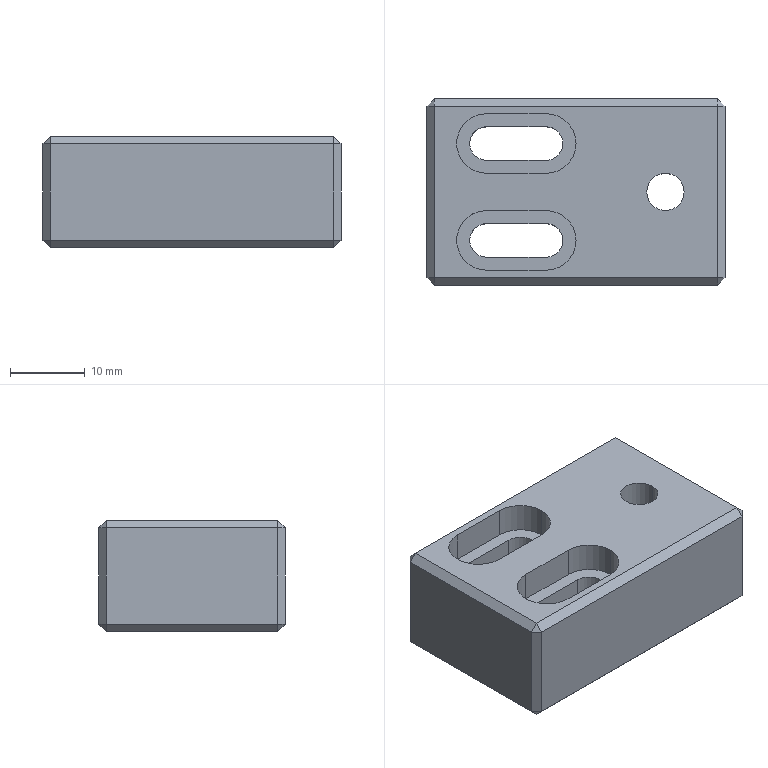Part | STEP file | 04-11 support stop post | 1 solid | 53 faces | box 40 x 25 x 15 mm | volume 11747 mm3 | plane 37 | cylinder 16 | commonest cylinder face diameters 4.5 x6 8 x6 5 x2 12 x2
STEP:
#1=CARTESIAN_POINT('',(-1.75,-6.5,0.));
#2=VERTEX_POINT('',#1);
#3=CARTESIAN_POINT('',(-4.,-4.25,0.));
#4=VERTEX_POINT('',#3);
#5=CARTESIAN_POINT('',(-4.,-6.5,0.));
#6=DIRECTION('',(0.,0.,1.));
#7=DIRECTION('',(1.,0.,0.));
#8=AXIS2_PLACEMENT_3D('',#5,#6,#7);
#9=CIRCLE('',#8,2.25);
#10=EDGE_CURVE('',#2,#4,#9,.T.);
#11=ORIENTED_EDGE('',*,*,#10,.F.);
#12=CARTESIAN_POINT('',(-1.75,-6.5,11.));
#13=VERTEX_POINT('',#12);
#14=CARTESIAN_POINT('',(-1.75,-6.5,-5.));
#15=DIRECTION('',(0.,0.,1.));
#16=VECTOR('',#15,1000.);
#17=LINE('',#14,#16);
#18=EDGE_CURVE('',#2,#13,#17,.T.);
#19=ORIENTED_EDGE('',*,*,#18,.T.);
#20=CARTESIAN_POINT('',(-4.,-4.25,11.));
#21=VERTEX_POINT('',#20);
#22=CARTESIAN_POINT('',(-4.,-6.5,11.));
#23=DIRECTION('',(0.,0.,1.));
#24=DIRECTION('',(-1.,0.,0.));
#25=AXIS2_PLACEMENT_3D('',#22,#23,#24);
#26=CIRCLE('',#25,2.25);
#27=EDGE_CURVE('',#13,#21,#26,.T.);
#28=ORIENTED_EDGE('',*,*,#27,.T.);
#29=CARTESIAN_POINT('',(-4.,-4.25,-5.));
#30=DIRECTION('',(0.,0.,1.));
#31=VECTOR('',#30,1000.);
#32=LINE('',#29,#31);
#33=EDGE_CURVE('',#4,#21,#32,.T.);
#34=ORIENTED_EDGE('',*,*,#33,.F.);
#35=EDGE_LOOP('',(#11,#19,#28,#34));
#36=FACE_OUTER_BOUND('',#35,.T.);
#37=CARTESIAN_POINT('',(-4.,-6.5,-5.));
#38=DIRECTION('',(0.,0.,1.));
#39=DIRECTION('',(1.,0.,0.));
#40=AXIS2_PLACEMENT_3D('',#37,#38,#39);
#41=CYLINDRICAL_SURFACE('',#40,2.25);
#42=ADVANCED_FACE('',(#36),#41,.F.);
#43=CARTESIAN_POINT('',(-1.75,6.5,0.));
#44=VERTEX_POINT('',#43);
#45=CARTESIAN_POINT('',(-4.,8.75,0.));
#46=VERTEX_POINT('',#45);
#47=CARTESIAN_POINT('',(-4.,6.5,0.));
#48=DIRECTION('',(0.,0.,1.));
#49=DIRECTION('',(1.,0.,0.));
#50=AXIS2_PLACEMENT_3D('',#47,#48,#49);
#51=CIRCLE('',#50,2.25);
#52=EDGE_CURVE('',#44,#46,#51,.T.);
#53=ORIENTED_EDGE('',*,*,#52,.F.);
#54=CARTESIAN_POINT('',(-1.75,6.5,11.));
#55=VERTEX_POINT('',#54);
#56=CARTESIAN_POINT('',(-1.75,6.5,-5.));
#57=DIRECTION('',(0.,0.,1.));
#58=VECTOR('',#57,1000.);
#59=LINE('',#56,#58);
#60=EDGE_CURVE('',#44,#55,#59,.T.);
#61=ORIENTED_EDGE('',*,*,#60,.T.);
#62=CARTESIAN_POINT('',(-4.,8.75,11.));
#63=VERTEX_POINT('',#62);
#64=CARTESIAN_POINT('',(-4.,6.5,11.));
#65=DIRECTION('',(0.,0.,1.));
#66=DIRECTION('',(1.,0.,0.));
#67=AXIS2_PLACEMENT_3D('',#64,#65,#66);
#68=CIRCLE('',#67,2.25);
#69=EDGE_CURVE('',#55,#63,#68,.T.);
#70=ORIENTED_EDGE('',*,*,#69,.T.);
#71=CARTESIAN_POINT('',(-4.,8.75,-5.));
#72=DIRECTION('',(0.,0.,1.));
#73=VECTOR('',#72,1000.);
#74=LINE('',#71,#73);
#75=EDGE_CURVE('',#46,#63,#74,.T.);
#76=ORIENTED_EDGE('',*,*,#75,.F.);
#77=EDGE_LOOP('',(#53,#61,#70,#76));
#78=FACE_OUTER_BOUND('',#77,.T.);
#79=CARTESIAN_POINT('',(-4.,6.5,-5.));
#80=DIRECTION('',(0.,0.,1.));
#81=DIRECTION('',(1.,0.,0.));
#82=AXIS2_PLACEMENT_3D('',#79,#80,#81);
#83=CYLINDRICAL_SURFACE('',#82,2.25);
#84=ADVANCED_FACE('',(#78),#83,.F.);
#85=CARTESIAN_POINT('',(0.,-6.5,11.));
#86=VERTEX_POINT('',#85);
#87=CARTESIAN_POINT('',(-4.,-2.5,11.));
#88=VERTEX_POINT('',#87);
#89=CARTESIAN_POINT('',(-4.,-6.5,11.));
#90=DIRECTION('',(0.,0.,1.));
#91=DIRECTION('',(-1.,0.,0.));
#92=AXIS2_PLACEMENT_3D('',#89,#90,#91);
#93=CIRCLE('',#92,4.);
#94=EDGE_CURVE('',#86,#88,#93,.T.);
#95=ORIENTED_EDGE('',*,*,#94,.F.);
#96=CARTESIAN_POINT('',(0.,-6.5,15.));
#97=VERTEX_POINT('',#96);
#98=CARTESIAN_POINT('',(0.,-6.5,11.));
#99=DIRECTION('',(0.,0.,1.));
#100=VECTOR('',#99,1000.);
#101=LINE('',#98,#100);
#102=EDGE_CURVE('',#86,#97,#101,.T.);
#103=ORIENTED_EDGE('',*,*,#102,.T.);
#104=CARTESIAN_POINT('',(-4.,-2.5,15.));
#105=VERTEX_POINT('',#104);
#106=CARTESIAN_POINT('',(-4.,-6.5,15.));
#107=DIRECTION('',(0.,0.,1.));
#108=DIRECTION('',(-1.,0.,0.));
#109=AXIS2_PLACEMENT_3D('',#106,#107,#108);
#110=CIRCLE('',#109,4.);
#111=EDGE_CURVE('',#97,#105,#110,.T.);
#112=ORIENTED_EDGE('',*,*,#111,.T.);
#113=CARTESIAN_POINT('',(-4.,-2.5,11.));
#114=DIRECTION('',(0.,0.,1.));
#115=VECTOR('',#114,1000.);
#116=LINE('',#113,#115);
#117=EDGE_CURVE('',#88,#105,#116,.T.);
#118=ORIENTED_EDGE('',*,*,#117,.F.);
#119=EDGE_LOOP('',(#95,#103,#112,#118));
#120=FACE_OUTER_BOUND('',#119,.T.);
#121=CARTESIAN_POINT('',(-4.,-6.5,11.));
#122=DIRECTION('',(0.,0.,1.));
#123=DIRECTION('',(1.,0.,0.));
#124=AXIS2_PLACEMENT_3D('',#121,#122,#123);
#125=CYLINDRICAL_SURFACE('',#124,4.);
#126=ADVANCED_FACE('',(#120),#125,.F.);
#127=CARTESIAN_POINT('',(0.,6.5,11.));
#128=VERTEX_POINT('',#127);
#129=CARTESIAN_POINT('',(-4.,10.5,11.));
#130=VERTEX_POINT('',#129);
#131=CARTESIAN_POINT('',(-4.,6.5,11.));
#132=DIRECTION('',(0.,0.,1.));
#133=DIRECTION('',(1.,0.,0.));
#134=AXIS2_PLACEMENT_3D('',#131,#132,#133);
#135=CIRCLE('',#134,4.);
#136=EDGE_CURVE('',#128,#130,#135,.T.);
#137=ORIENTED_EDGE('',*,*,#136,.F.);
#138=CARTESIAN_POINT('',(0.,6.5,15.));
#139=VERTEX_POINT('',#138);
#140=CARTESIAN_POINT('',(0.,6.5,11.));
#141=DIRECTION('',(0.,0.,1.));
#142=VECTOR('',#141,1000.);
#143=LINE('',#140,#142);
#144=EDGE_CURVE('',#128,#139,#143,.T.);
#145=ORIENTED_EDGE('',*,*,#144,.T.);
#146=CARTESIAN_POINT('',(-4.,10.5,15.));
#147=VERTEX_POINT('',#146);
#148=CARTESIAN_POINT('',(-4.,6.5,15.));
#149=DIRECTION('',(0.,0.,1.));
#150=DIRECTION('',(1.,0.,0.));
#151=AXIS2_PLACEMENT_3D('',#148,#149,#150);
#152=CIRCLE('',#151,4.);
#153=EDGE_CURVE('',#139,#147,#152,.T.);
#154=ORIENTED_EDGE('',*,*,#153,.T.);
#155=CARTESIAN_POINT('',(-4.,10.5,11.));
#156=DIRECTION('',(0.,0.,1.));
#157=VECTOR('',#156,1000.);
#158=LINE('',#155,#157);
#159=EDGE_CURVE('',#130,#147,#158,.T.);
#160=ORIENTED_EDGE('',*,*,#159,.F.);
#161=EDGE_LOOP('',(#137,#145,#154,#160));
#162=FACE_OUTER_BOUND('',#161,.T.);
#163=CARTESIAN_POINT('',(-4.,6.5,11.));
#164=DIRECTION('',(0.,0.,1.));
#165=DIRECTION('',(1.,0.,0.));
#166=AXIS2_PLACEMENT_3D('',#163,#164,#165);
#167=CYLINDRICAL_SURFACE('',#166,4.);
#168=ADVANCED_FACE('',(#162),#167,.F.);
#169=CARTESIAN_POINT('',(18.,0.,8.));
#170=VERTEX_POINT('',#169);
#171=CARTESIAN_POINT('',(6.,0.,8.));
#172=VERTEX_POINT('',#171);
#173=CARTESIAN_POINT('',(12.,0.,8.));
#174=DIRECTION('',(0.,0.,-1.));
#175=DIRECTION('',(-1.,0.,0.));
#176=AXIS2_PLACEMENT_3D('',#173,#174,#175);
#177=CIRCLE('',#176,6.);
#178=EDGE_CURVE('',#170,#172,#177,.T.);
#179=ORIENTED_EDGE('',*,*,#178,.F.);
#180=CARTESIAN_POINT('',(18.,0.,0.));
#181=VERTEX_POINT('',#180);
#182=CARTESIAN_POINT('',(18.,0.,8.));
#183=DIRECTION('',(0.,0.,-1.));
#184=VECTOR('',#183,1000.);
#185=LINE('',#182,#184);
#186=EDGE_CURVE('',#170,#181,#185,.T.);
#187=ORIENTED_EDGE('',*,*,#186,.T.);
#188=CARTESIAN_POINT('',(6.,0.,0.));
#189=VERTEX_POINT('',#188);
#190=CARTESIAN_POINT('',(12.,0.,0.));
#191=DIRECTION('',(0.,0.,-1.));
#192=DIRECTION('',(-1.,0.,0.));
#193=AXIS2_PLACEMENT_3D('',#190,#191,#192);
#194=CIRCLE('',#193,6.);
#195=EDGE_CURVE('',#181,#189,#194,.T.);
#196=ORIENTED_EDGE('',*,*,#195,.T.);
#197=CARTESIAN_POINT('',(6.,0.,8.));
#198=DIRECTION('',(0.,0.,-1.));
#199=VECTOR('',#198,1000.);
#200=LINE('',#197,#199);
#201=EDGE_CURVE('',#172,#189,#200,.T.);
#202=ORIENTED_EDGE('',*,*,#201,.F.);
#203=EDGE_LOOP('',(#179,#187,#196,#202));
#204=FACE_OUTER_BOUND('',#203,.T.);
#205=CARTESIAN_POINT('',(12.,0.,8.));
#206=DIRECTION('',(0.,0.,-1.));
#207=DIRECTION('',(-1.,0.,0.));
#208=AXIS2_PLACEMENT_3D('',#205,#206,#207);
#209=CYLINDRICAL_SURFACE('',#208,6.);
#210=ADVANCED_FACE('',(#204),#209,.F.);
#211=CARTESIAN_POINT('',(9.5,0.,8.));
#212=VERTEX_POINT('',#211);
#213=CARTESIAN_POINT('',(14.5,0.,8.));
#214=VERTEX_POINT('',#213);
#215=CARTESIAN_POINT('',(12.,0.,8.));
#216=DIRECTION('',(0.,0.,1.));
#217=DIRECTION('',(-1.,0.,0.));
#218=AXIS2_PLACEMENT_3D('',#215,#216,#217);
#219=CIRCLE('',#218,2.5);
#220=EDGE_CURVE('',#212,#214,#219,.T.);
#221=ORIENTED_EDGE('',*,*,#220,.F.);
#222=CARTESIAN_POINT('',(9.5,0.,15.));
#223=VERTEX_POINT('',#222);
#224=CARTESIAN_POINT('',(9.5,0.,-2.));
#225=DIRECTION('',(0.,0.,1.));
#226=VECTOR('',#225,1000.);
#227=LINE('',#224,#226);
#228=EDGE_CURVE('',#212,#223,#227,.T.);
#229=ORIENTED_EDGE('',*,*,#228,.T.);
#230=CARTESIAN_POINT('',(14.5,0.,15.));
#231=VERTEX_POINT('',#230);
#232=CARTESIAN_POINT('',(12.,0.,15.));
#233=DIRECTION('',(0.,0.,1.));
#234=DIRECTION('',(1.,0.,0.));
#235=AXIS2_PLACEMENT_3D('',#232,#233,#234);
#236=CIRCLE('',#235,2.5);
#237=EDGE_CURVE('',#223,#231,#236,.T.);
#238=ORIENTED_EDGE('',*,*,#237,.T.);
#239=CARTESIAN_POINT('',(14.5,0.,-2.));
#240=DIRECTION('',(0.,0.,1.));
#241=VECTOR('',#240,1000.);
#242=LINE('',#239,#241);
#243=EDGE_CURVE('',#214,#231,#242,.T.);
#244=ORIENTED_EDGE('',*,*,#243,.F.);
#245=EDGE_LOOP('',(#221,#229,#238,#244));
#246=FACE_OUTER_BOUND('',#245,.T.);
#247=CARTESIAN_POINT('',(12.,0.,-2.));
#248=DIRECTION('',(0.,0.,1.));
#249=DIRECTION('',(1.,0.,0.));
#250=AXIS2_PLACEMENT_3D('',#247,#248,#249);
#251=CYLINDRICAL_SURFACE('',#250,2.5);
#252=ADVANCED_FACE('',(#246),#251,.F.);
#253=ORIENTED_EDGE('',*,*,#228,.F.);
#254=CARTESIAN_POINT('',(12.,0.,8.));
#255=DIRECTION('',(0.,0.,1.));
#256=DIRECTION('',(-1.,0.,0.));
#257=AXIS2_PLACEMENT_3D('',#254,#255,#256);
#258=CIRCLE('',#257,2.5);
#259=EDGE_CURVE('',#214,#212,#258,.T.);
#260=ORIENTED_EDGE('',*,*,#259,.F.);
#261=ORIENTED_EDGE('',*,*,#243,.T.);
#262=CARTESIAN_POINT('',(12.,0.,15.));
#263=DIRECTION('',(0.,0.,1.));
#264=DIRECTION('',(1.,0.,0.));
#265=AXIS2_PLACEMENT_3D('',#262,#263,#264);
#266=CIRCLE('',#265,2.5);
#267=EDGE_CURVE('',#231,#223,#266,.T.);
#268=ORIENTED_EDGE('',*,*,#267,.T.);
#269=EDGE_LOOP('',(#253,#260,#261,#268));
#270=FACE_OUTER_BOUND('',#269,.T.);
#271=CARTESIAN_POINT('',(12.,0.,-2.));
#272=DIRECTION('',(0.,0.,1.));
#273=DIRECTION('',(1.,0.,0.));
#274=AXIS2_PLACEMENT_3D('',#271,#272,#273);
#275=CYLINDRICAL_SURFACE('',#274,2.5);
#276=ADVANCED_FACE('',(#270),#275,.F.);
#277=CARTESIAN_POINT('',(20.,11.5,14.));
#278=VERTEX_POINT('',#277);
#279=CARTESIAN_POINT('',(20.,-11.5,14.));
#280=VERTEX_POINT('',#279);
#281=CARTESIAN_POINT('',(20.,-12.5,14.));
#282=DIRECTION('',(0.,-1.,0.));
#283=VECTOR('',#282,1000.);
#284=LINE('',#281,#283);
#285=EDGE_CURVE('',#278,#280,#284,.T.);
#286=ORIENTED_EDGE('',*,*,#285,.T.);
#287=CARTESIAN_POINT('',(20.,-11.5,1.));
#288=VERTEX_POINT('',#287);
#289=CARTESIAN_POINT('',(20.,-11.5,15.));
#290=DIRECTION('',(0.,0.,-1.));
#291=VECTOR('',#290,1000.);
#292=LINE('',#289,#291);
#293=EDGE_CURVE('',#280,#288,#292,.T.);
#294=ORIENTED_EDGE('',*,*,#293,.T.);
#295=CARTESIAN_POINT('',(20.,11.5,1.));
#296=VERTEX_POINT('',#295);
#297=CARTESIAN_POINT('',(20.,12.5,1.));
#298=DIRECTION('',(0.,1.,0.));
#299=VECTOR('',#298,1000.);
#300=LINE('',#297,#299);
#301=EDGE_CURVE('',#288,#296,#300,.T.);
#302=ORIENTED_EDGE('',*,*,#301,.T.);
#303=CARTESIAN_POINT('',(20.,11.5,15.));
#304=DIRECTION('',(0.,0.,1.));
#305=VECTOR('',#304,1000.);
#306=LINE('',#303,#305);
#307=EDGE_CURVE('',#296,#278,#306,.T.);
#308=ORIENTED_EDGE('',*,*,#307,.T.);
#309=EDGE_LOOP('',(#286,#294,#302,#308));
#310=FACE_OUTER_BOUND('',#309,.T.);
#311=CARTESIAN_POINT('',(20.,12.5,15.));
#312=DIRECTION('',(-1.,0.,0.));
#313=DIRECTION('',(0.,-1.,0.));
#314=AXIS2_PLACEMENT_3D('',#311,#312,#313);
#315=PLANE('',#314);
#316=ADVANCED_FACE('',(#310),#315,.F.);
#317=CARTESIAN_POINT('',(19.,12.5,14.));
#318=VERTEX_POINT('',#317);
#319=CARTESIAN_POINT('',(19.,12.5,1.));
#320=VERTEX_POINT('',#319);
#321=CARTESIAN_POINT('',(19.,12.5,15.));
#322=DIRECTION('',(0.,0.,-1.));
#323=VECTOR('',#322,1000.);
#324=LINE('',#321,#323);
#325=EDGE_CURVE('',#318,#320,#324,.T.);
#326=ORIENTED_EDGE('',*,*,#325,.T.);
#327=CARTESIAN_POINT('',(-19.,12.5,1.));
#328=VERTEX_POINT('',#327);
#329=CARTESIAN_POINT('',(-20.,12.5,1.));
#330=DIRECTION('',(-1.,0.,0.));
#331=VECTOR('',#330,1000.);
#332=LINE('',#329,#331);
#333=EDGE_CURVE('',#320,#328,#332,.T.);
#334=ORIENTED_EDGE('',*,*,#333,.T.);
#335=CARTESIAN_POINT('',(-19.,12.5,14.));
#336=VERTEX_POINT('',#335);
#337=CARTESIAN_POINT('',(-19.,12.5,15.));
#338=DIRECTION('',(0.,0.,1.));
#339=VECTOR('',#338,1000.);
#340=LINE('',#337,#339);
#341=EDGE_CURVE('',#328,#336,#340,.T.);
#342=ORIENTED_EDGE('',*,*,#341,.T.);
#343=CARTESIAN_POINT('',(20.,12.5,14.));
#344=DIRECTION('',(1.,0.,0.));
#345=VECTOR('',#344,1000.);
#346=LINE('',#343,#345);
#347=EDGE_CURVE('',#336,#318,#346,.T.);
#348=ORIENTED_EDGE('',*,*,#347,.T.);
#349=EDGE_LOOP('',(#326,#334,#342,#348));
#350=FACE_OUTER_BOUND('',#349,.T.);
#351=CARTESIAN_POINT('',(-20.,12.5,15.));
#352=DIRECTION('',(0.,-1.,0.));
#353=DIRECTION('',(0.,0.,-1.));
#354=AXIS2_PLACEMENT_3D('',#351,#352,#353);
#355=PLANE('',#354);
#356=ADVANCED_FACE('',(#350),#355,.F.);
#357=CARTESIAN_POINT('',(-20.,11.5,14.));
#358=VERTEX_POINT('',#357);
#359=CARTESIAN_POINT('',(-20.,11.5,1.));
#360=VERTEX_POINT('',#359);
#361=CARTESIAN_POINT('',(-20.,11.5,15.));
#362=DIRECTION('',(0.,0.,-1.));
#363=VECTOR('',#362,1000.);
#364=LINE('',#361,#363);
#365=EDGE_CURVE('',#358,#360,#364,.T.);
#366=ORIENTED_EDGE('',*,*,#365,.T.);
#367=CARTESIAN_POINT('',(-20.,-11.5,1.));
#368=VERTEX_POINT('',#367);
#369=CARTESIAN_POINT('',(-20.,12.5,1.));
#370=DIRECTION('',(0.,-1.,0.));
#371=VECTOR('',#370,1000.);
#372=LINE('',#369,#371);
#373=EDGE_CURVE('',#360,#368,#372,.T.);
#374=ORIENTED_EDGE('',*,*,#373,.T.);
#375=CARTESIAN_POINT('',(-20.,-11.5,14.));
#376=VERTEX_POINT('',#375);
#377=CARTESIAN_POINT('',(-20.,-11.5,15.));
#378=DIRECTION('',(0.,0.,1.));
#379=VECTOR('',#378,1000.);
#380=LINE('',#377,#379);
#381=EDGE_CURVE('',#368,#376,#380,.T.);
#382=ORIENTED_EDGE('',*,*,#381,.T.);
#383=CARTESIAN_POINT('',(-20.,12.5,14.));
#384=DIRECTION('',(0.,1.,0.));
#385=VECTOR('',#384,1000.);
#386=LINE('',#383,#385);
#387=EDGE_CURVE('',#376,#358,#386,.T.);
#388=ORIENTED_EDGE('',*,*,#387,.T.);
#389=EDGE_LOOP('',(#366,#374,#382,#388));
#390=FACE_OUTER_BOUND('',#389,.T.);
#391=CARTESIAN_POINT('',(-20.,12.5,15.));
#392=DIRECTION('',(1.,0.,0.));
#393=DIRECTION('',(0.,1.,0.));
#394=AXIS2_PLACEMENT_3D('',#391,#392,#393);
#395=PLANE('',#394);
#396=ADVANCED_FACE('',(#390),#395,.F.);
#397=CARTESIAN_POINT('',(19.,-12.5,1.));
#398=VERTEX_POINT('',#397);
#399=CARTESIAN_POINT('',(19.,-12.5,14.));
#400=VERTEX_POINT('',#399);
#401=CARTESIAN_POINT('',(19.,-12.5,15.));
#402=DIRECTION('',(0.,0.,1.));
#403=VECTOR('',#402,1000.);
#404=LINE('',#401,#403);
#405=EDGE_CURVE('',#398,#400,#404,.T.);
#406=ORIENTED_EDGE('',*,*,#405,.T.);
#407=CARTESIAN_POINT('',(-19.,-12.5,14.));
#408=VERTEX_POINT('',#407);
#409=CARTESIAN_POINT('',(-20.,-12.5,14.));
#410=DIRECTION('',(-1.,0.,0.));
#411=VECTOR('',#410,1000.);
#412=LINE('',#409,#411);
#413=EDGE_CURVE('',#400,#408,#412,.T.);
#414=ORIENTED_EDGE('',*,*,#413,.T.);
#415=CARTESIAN_POINT('',(-19.,-12.5,1.));
#416=VERTEX_POINT('',#415);
#417=CARTESIAN_POINT('',(-19.,-12.5,15.));
#418=DIRECTION('',(0.,0.,-1.));
#419=VECTOR('',#418,1000.);
#420=LINE('',#417,#419);
#421=EDGE_CURVE('',#408,#416,#420,.T.);
#422=ORIENTED_EDGE('',*,*,#421,.T.);
#423=CARTESIAN_POINT('',(-20.,-12.5,1.));
#424=DIRECTION('',(1.,0.,0.));
#425=VECTOR('',#424,1000.);
#426=LINE('',#423,#425);
#427=EDGE_CURVE('',#416,#398,#426,.T.);
#428=ORIENTED_EDGE('',*,*,#427,.T.);
#429=EDGE_LOOP('',(#406,#414,#422,#428));
#430=FACE_OUTER_BOUND('',#429,.T.);
#431=CARTESIAN_POINT('',(-20.,-12.5,15.));
#432=DIRECTION('',(0.,1.,0.));
#433=DIRECTION('',(0.,0.,1.));
#434=AXIS2_PLACEMENT_3D('',#431,#432,#433);
#435=PLANE('',#434);
#436=ADVANCED_FACE('',(#430),#435,.F.);
#437=CARTESIAN_POINT('',(-19.,11.5,15.));
#438=VERTEX_POINT('',#437);
#439=CARTESIAN_POINT('',(-19.,-11.5,15.));
#440=VERTEX_POINT('',#439);
#441=CARTESIAN_POINT('',(-19.,-12.5,15.));
#442=DIRECTION('',(0.,-1.,0.));
#443=VECTOR('',#442,1000.);
#444=LINE('',#441,#443);
#445=EDGE_CURVE('',#438,#440,#444,.T.);
#446=ORIENTED_EDGE('',*,*,#445,.T.);
#447=CARTESIAN_POINT('',(19.,-11.5,15.));
#448=VERTEX_POINT('',#447);
#449=CARTESIAN_POINT('',(20.,-11.5,15.));
#450=DIRECTION('',(1.,0.,0.));
#451=VECTOR('',#450,1000.);
#452=LINE('',#449,#451);
#453=EDGE_CURVE('',#440,#448,#452,.T.);
#454=ORIENTED_EDGE('',*,*,#453,.T.);
#455=CARTESIAN_POINT('',(19.,11.5,15.));
#456=VERTEX_POINT('',#455);
#457=CARTESIAN_POINT('',(19.,12.5,15.));
#458=DIRECTION('',(0.,1.,0.));
#459=VECTOR('',#458,1000.);
#460=LINE('',#457,#459);
#461=EDGE_CURVE('',#448,#456,#460,.T.);
#462=ORIENTED_EDGE('',*,*,#461,.T.);
#463=CARTESIAN_POINT('',(-20.,11.5,15.));
#464=DIRECTION('',(-1.,0.,0.));
#465=VECTOR('',#464,1000.);
#466=LINE('',#463,#465);
#467=EDGE_CURVE('',#456,#438,#466,.T.);
#468=ORIENTED_EDGE('',*,*,#467,.T.);
#469=EDGE_LOOP('',(#446,#454,#462,#468));
#470=FACE_OUTER_BOUND('',#469,.T.);
#471=CARTESIAN_POINT('',(-12.,-2.5,15.));
#472=VERTEX_POINT('',#471);
#473=CARTESIAN_POINT('',(-12.,-10.5,15.));
#474=VERTEX_POINT('',#473);
#475=CARTESIAN_POINT('',(-12.,-6.5,15.));
#476=DIRECTION('',(0.,0.,1.));
#477=DIRECTION('',(-1.,0.,0.));
#478=AXIS2_PLACEMENT_3D('',#475,#476,#477);
#479=CIRCLE('',#478,4.);
#480=EDGE_CURVE('',#472,#474,#479,.T.);
#481=ORIENTED_EDGE('',*,*,#480,.F.);
#482=CARTESIAN_POINT('',(-12.,-2.5,15.));
#483=DIRECTION('',(-1.,0.,0.));
#484=VECTOR('',#483,1000.);
#485=LINE('',#482,#484);
#486=EDGE_CURVE('',#105,#472,#485,.T.);
#487=ORIENTED_EDGE('',*,*,#486,.F.);
#488=ORIENTED_EDGE('',*,*,#111,.F.);
#489=CARTESIAN_POINT('',(-4.,-10.5,15.));
#490=VERTEX_POINT('',#489);
#491=CARTESIAN_POINT('',(-4.,-6.5,15.));
#492=DIRECTION('',(0.,0.,1.));
#493=DIRECTION('',(-1.,0.,0.));
#494=AXIS2_PLACEMENT_3D('',#491,#492,#493);
#495=CIRCLE('',#494,4.);
#496=EDGE_CURVE('',#490,#97,#495,.T.);
#497=ORIENTED_EDGE('',*,*,#496,.F.);
#498=CARTESIAN_POINT('',(-12.,-10.5,15.));
#499=DIRECTION('',(1.,0.,0.));
#500=VECTOR('',#499,1000.);
#501=LINE('',#498,#500);
#502=EDGE_CURVE('',#474,#490,#501,.T.);
#503=ORIENTED_EDGE('',*,*,#502,.F.);
#504=EDGE_LOOP('',(#481,#487,#488,#497,#503));
#505=FACE_BOUND('',#504,.T.);
#506=CARTESIAN_POINT('',(-12.,10.5,15.));
#507=VERTEX_POINT('',#506);
#508=CARTESIAN_POINT('',(-12.,2.5,15.));
#509=VERTEX_POINT('',#508);
#510=CARTESIAN_POINT('',(-12.,6.5,15.));
#511=DIRECTION('',(0.,0.,1.));
#512=DIRECTION('',(1.,0.,0.));
#513=AXIS2_PLACEMENT_3D('',#510,#511,#512);
#514=CIRCLE('',#513,4.);
#515=EDGE_CURVE('',#507,#509,#514,.T.);
#516=ORIENTED_EDGE('',*,*,#515,.F.);
#517=CARTESIAN_POINT('',(-12.,10.5,15.));
#518=DIRECTION('',(-1.,0.,0.));
#519=VECTOR('',#518,1000.);
#520=LINE('',#517,#519);
#521=EDGE_CURVE('',#147,#507,#520,.T.);
#522=ORIENTED_EDGE('',*,*,#521,.F.);
#523=ORIENTED_EDGE('',*,*,#153,.F.);
#524=CARTESIAN_POINT('',(-4.,2.5,15.));
#525=VERTEX_POINT('',#524);
#526=CARTESIAN_POINT('',(-4.,6.5,15.));
#527=DIRECTION('',(0.,0.,1.));
#528=DIRECTION('',(1.,0.,0.));
#529=AXIS2_PLACEMENT_3D('',#526,#527,#528);
#530=CIRCLE('',#529,4.);
#531=EDGE_CURVE('',#525,#139,#530,.T.);
#532=ORIENTED_EDGE('',*,*,#531,.F.);
#533=CARTESIAN_POINT('',(-12.,2.5,15.));
#534=DIRECTION('',(1.,0.,0.));
#535=VECTOR('',#534,1000.);
#536=LINE('',#533,#535);
#537=EDGE_CURVE('',#509,#525,#536,.T.);
#538=ORIENTED_EDGE('',*,*,#537,.F.);
#539=EDGE_LOOP('',(#516,#522,#523,#532,#538));
#540=FACE_BOUND('',#539,.T.);
#541=ORIENTED_EDGE('',*,*,#267,.F.);
#542=ORIENTED_EDGE('',*,*,#237,.F.);
#543=EDGE_LOOP('',(#541,#542));
#544=FACE_BOUND('',#543,.T.);
#545=CARTESIAN_POINT('',(20.,-12.5,15.));
#546=DIRECTION('',(0.,0.,1.));
#547=DIRECTION('',(1.,0.,0.));
#548=AXIS2_PLACEMENT_3D('',#545,#546,#547);
#549=PLANE('',#548);
#550=ADVANCED_FACE('',(#470,#505,#540,#544),#549,.T.);
#551=CARTESIAN_POINT('',(19.,11.5,0.));
#552=VERTEX_POINT('',#551);
#553=CARTESIAN_POINT('',(19.,-11.5,0.));
#554=VERTEX_POINT('',#553);
#555=CARTESIAN_POINT('',(19.,-12.5,0.));
#556=DIRECTION('',(0.,-1.,0.));
#557=VECTOR('',#556,1000.);
#558=LINE('',#555,#557);
#559=EDGE_CURVE('',#552,#554,#558,.T.);
#560=ORIENTED_EDGE('',*,*,#559,.T.);
#561=CARTESIAN_POINT('',(-19.,-11.5,0.));
#562=VERTEX_POINT('',#561);
#563=CARTESIAN_POINT('',(20.,-11.5,0.));
#564=DIRECTION('',(-1.,0.,0.));
#565=VECTOR('',#564,1000.);
#566=LINE('',#563,#565);
#567=EDGE_CURVE('',#554,#562,#566,.T.);
#568=ORIENTED_EDGE('',*,*,#567,.T.);
#569=CARTESIAN_POINT('',(-19.,11.5,0.));
#570=VERTEX_POINT('',#569);
#571=CARTESIAN_POINT('',(-19.,-12.5,0.));
#572=DIRECTION('',(0.,1.,0.));
#573=VECTOR('',#572,1000.);
#574=LINE('',#571,#573);
#575=EDGE_CURVE('',#562,#570,#574,.T.);
#576=ORIENTED_EDGE('',*,*,#575,.T.);
#577=CARTESIAN_POINT('',(20.,11.5,0.));
#578=DIRECTION('',(1.,0.,0.));
#579=VECTOR('',#578,1000.);
#580=LINE('',#577,#579);
#581=EDGE_CURVE('',#570,#552,#580,.T.);
#582=ORIENTED_EDGE('',*,*,#581,.T.);
#583=EDGE_LOOP('',(#560,#568,#576,#582));
#584=FACE_OUTER_BOUND('',#583,.T.);
#585=CARTESIAN_POINT('',(-12.,-4.25,0.));
#586=VERTEX_POINT('',#585);
#587=CARTESIAN_POINT('',(20.,-4.25,0.));
#588=DIRECTION('',(-1.,0.,0.));
#589=VECTOR('',#588,1000.);
#590=LINE('',#587,#589);
#591=EDGE_CURVE('',#4,#586,#590,.T.);
#592=ORIENTED_EDGE('',*,*,#591,.T.);
#593=CARTESIAN_POINT('',(-12.,-8.75,0.));
#594=VERTEX_POINT('',#593);
#595=CARTESIAN_POINT('',(-12.,-6.5,0.));
#596=DIRECTION('',(0.,0.,1.));
#597=DIRECTION('',(1.,0.,0.));
#598=AXIS2_PLACEMENT_3D('',#595,#596,#597);
#599=CIRCLE('',#598,2.25);
#600=EDGE_CURVE('',#586,#594,#599,.T.);
#601=ORIENTED_EDGE('',*,*,#600,.T.);
#602=CARTESIAN_POINT('',(-4.,-8.75,0.));
#603=VERTEX_POINT('',#602);
#604=CARTESIAN_POINT('',(20.,-8.75,0.));
#605=DIRECTION('',(1.,0.,0.));
#606=VECTOR('',#605,1000.);
#607=LINE('',#604,#606);
#608=EDGE_CURVE('',#594,#603,#607,.T.);
#609=ORIENTED_EDGE('',*,*,#608,.T.);
#610=CARTESIAN_POINT('',(-4.,-6.5,0.));
#611=DIRECTION('',(0.,0.,1.));
#612=DIRECTION('',(1.,0.,0.));
#613=AXIS2_PLACEMENT_3D('',#610,#611,#612);
#614=CIRCLE('',#613,2.25);
#615=EDGE_CURVE('',#603,#2,#614,.T.);
#616=ORIENTED_EDGE('',*,*,#615,.T.);
#617=ORIENTED_EDGE('',*,*,#10,.T.);
#618=EDGE_LOOP('',(#592,#601,#609,#616,#617));
#619=FACE_BOUND('',#618,.T.);
#620=CARTESIAN_POINT('',(-12.,8.75,0.));
#621=VERTEX_POINT('',#620);
#622=CARTESIAN_POINT('',(20.,8.75,0.));
#623=DIRECTION('',(-1.,0.,0.));
#624=VECTOR('',#623,1000.);
#625=LINE('',#622,#624);
#626=EDGE_CURVE('',#46,#621,#625,.T.);
#627=ORIENTED_EDGE('',*,*,#626,.T.);
#628=CARTESIAN_POINT('',(-12.,4.25,0.));
#629=VERTEX_POINT('',#628);
#630=CARTESIAN_POINT('',(-12.,6.5,0.));
#631=DIRECTION('',(0.,0.,1.));
#632=DIRECTION('',(1.,0.,0.));
#633=AXIS2_PLACEMENT_3D('',#630,#631,#632);
#634=CIRCLE('',#633,2.25);
#635=EDGE_CURVE('',#621,#629,#634,.T.);
#636=ORIENTED_EDGE('',*,*,#635,.T.);
#637=CARTESIAN_POINT('',(-4.,4.25,0.));
#638=VERTEX_POINT('',#637);
#639=CARTESIAN_POINT('',(20.,4.25,0.));
#640=DIRECTION('',(1.,0.,0.));
#641=VECTOR('',#640,1000.);
#642=LINE('',#639,#641);
#643=EDGE_CURVE('',#629,#638,#642,.T.);
#644=ORIENTED_EDGE('',*,*,#643,.T.);
#645=CARTESIAN_POINT('',(-4.,6.5,0.));
#646=DIRECTION('',(0.,0.,1.));
#647=DIRECTION('',(1.,0.,0.));
#648=AXIS2_PLACEMENT_3D('',#645,#646,#647);
#649=CIRCLE('',#648,2.25);
#650=EDGE_CURVE('',#638,#44,#649,.T.);
#651=ORIENTED_EDGE('',*,*,#650,.T.);
#652=ORIENTED_EDGE('',*,*,#52,.T.);
#653=EDGE_LOOP('',(#627,#636,#644,#651,#652));
#654=FACE_BOUND('',#653,.T.);
#655=CARTESIAN_POINT('',(12.,0.,0.));
#656=DIRECTION('',(0.,0.,-1.));
#657=DIRECTION('',(-1.,0.,0.));
#658=AXIS2_PLACEMENT_3D('',#655,#656,#657);
#659=CIRCLE('',#658,6.);
#660=EDGE_CURVE('',#189,#181,#659,.T.);
#661=ORIENTED_EDGE('',*,*,#660,.F.);
#662=ORIENTED_EDGE('',*,*,#195,.F.);
#663=EDGE_LOOP('',(#661,#662));
#664=FACE_BOUND('',#663,.T.);
#665=CARTESIAN_POINT('',(20.,-12.5,0.));
#666=DIRECTION('',(0.,0.,1.));
#667=DIRECTION('',(1.,0.,0.));
#668=AXIS2_PLACEMENT_3D('',#665,#666,#667);
#669=PLANE('',#668);
#670=ADVANCED_FACE('',(#584,#619,#654,#664),#669,.F.);
#671=CARTESIAN_POINT('',(12.,0.,8.));
#672=DIRECTION('',(0.,0.,-1.));
#673=DIRECTION('',(-1.,0.,0.));
#674=AXIS2_PLACEMENT_3D('',#671,#672,#673);
#675=CIRCLE('',#674,6.);
#676=EDGE_CURVE('',#172,#170,#675,.T.);
#677=ORIENTED_EDGE('',*,*,#676,.T.);
#678=ORIENTED_EDGE('',*,*,#178,.T.);
#679=EDGE_LOOP('',(#677,#678));
#680=FACE_OUTER_BOUND('',#679,.T.);
#681=ORIENTED_EDGE('',*,*,#259,.T.);
#682=ORIENTED_EDGE('',*,*,#220,.T.);
#683=EDGE_LOOP('',(#681,#682));
#684=FACE_BOUND('',#683,.T.);
#685=CARTESIAN_POINT('',(12.,0.,8.));
#686=DIRECTION('',(0.,0.,-1.));
#687=DIRECTION('',(-1.,0.,0.));
#688=AXIS2_PLACEMENT_3D('',#685,#686,#687);
#689=PLANE('',#688);
#690=ADVANCED_FACE('',(#680,#684),#689,.T.);
#691=ORIENTED_EDGE('',*,*,#186,.F.);
#692=ORIENTED_EDGE('',*,*,#676,.F.);
#693=ORIENTED_EDGE('',*,*,#201,.T.);
#694=ORIENTED_EDGE('',*,*,#660,.T.);
#695=EDGE_LOOP('',(#691,#692,#693,#694));
#696=FACE_OUTER_BOUND('',#695,.T.);
#697=CARTESIAN_POINT('',(12.,0.,8.));
#698=DIRECTION('',(0.,0.,-1.));
#699=DIRECTION('',(-1.,0.,0.));
#700=AXIS2_PLACEMENT_3D('',#697,#698,#699);
#701=CYLINDRICAL_SURFACE('',#700,6.);
#702=ADVANCED_FACE('',(#696),#701,.F.);
#703=ORIENTED_EDGE('',*,*,#515,.T.);
#704=CARTESIAN_POINT('',(-12.,2.5,11.));
#705=VERTEX_POINT('',#704);
#706=CARTESIAN_POINT('',(-12.,2.5,11.));
#707=DIRECTION('',(0.,0.,1.));
#708=VECTOR('',#707,1000.);
#709=LINE('',#706,#708);
#710=EDGE_CURVE('',#705,#509,#709,.T.);
#711=ORIENTED_EDGE('',*,*,#710,.F.);
#712=CARTESIAN_POINT('',(-12.,10.5,11.));
#713=VERTEX_POINT('',#712);
#714=CARTESIAN_POINT('',(-12.,6.5,11.));
#715=DIRECTION('',(0.,0.,1.));
#716=DIRECTION('',(1.,0.,0.));
#717=AXIS2_PLACEMENT_3D('',#714,#715,#716);
#718=CIRCLE('',#717,4.);
#719=EDGE_CURVE('',#713,#705,#718,.T.);
#720=ORIENTED_EDGE('',*,*,#719,.F.);
#721=CARTESIAN_POINT('',(-12.,10.5,11.));
#722=DIRECTION('',(0.,0.,1.));
#723=VECTOR('',#722,1000.);
#724=LINE('',#721,#723);
#725=EDGE_CURVE('',#713,#507,#724,.T.);
#726=ORIENTED_EDGE('',*,*,#725,.T.);
#727=EDGE_LOOP('',(#703,#711,#720,#726));
#728=FACE_OUTER_BOUND('',#727,.T.);
#729=CARTESIAN_POINT('',(-12.,6.5,11.));
#730=DIRECTION('',(0.,0.,1.));
#731=DIRECTION('',(1.,0.,0.));
#732=AXIS2_PLACEMENT_3D('',#729,#730,#731);
#733=CYLINDRICAL_SURFACE('',#732,4.);
#734=ADVANCED_FACE('',(#728),#733,.F.);
#735=ORIENTED_EDGE('',*,*,#521,.T.);
#736=ORIENTED_EDGE('',*,*,#725,.F.);
#737=CARTESIAN_POINT('',(-12.,10.5,11.));
#738=DIRECTION('',(-1.,0.,0.));
#739=VECTOR('',#738,1000.);
#740=LINE('',#737,#739);
#741=EDGE_CURVE('',#130,#713,#740,.T.);
#742=ORIENTED_EDGE('',*,*,#741,.F.);
#743=ORIENTED_EDGE('',*,*,#159,.T.);
#744=EDGE_LOOP('',(#735,#736,#742,#743));
#745=FACE_OUTER_BOUND('',#744,.T.);
#746=CARTESIAN_POINT('',(-12.,10.5,11.));
#747=DIRECTION('',(0.,1.,0.));
#748=DIRECTION('',(0.,0.,1.));
#749=AXIS2_PLACEMENT_3D('',#746,#747,#748);
#750=PLANE('',#749);
#751=ADVANCED_FACE('',(#745),#750,.F.);
#752=ORIENTED_EDGE('',*,*,#144,.F.);
#753=CARTESIAN_POINT('',(-4.,2.5,11.));
#754=VERTEX_POINT('',#753);
#755=CARTESIAN_POINT('',(-4.,6.5,11.));
#756=DIRECTION('',(0.,0.,1.));
#757=DIRECTION('',(1.,0.,0.));
#758=AXIS2_PLACEMENT_3D('',#755,#756,#757);
#759=CIRCLE('',#758,4.);
#760=EDGE_CURVE('',#754,#128,#759,.T.);
#761=ORIENTED_EDGE('',*,*,#760,.F.);
#762=CARTESIAN_POINT('',(-4.,2.5,11.));
#763=DIRECTION('',(0.,0.,1.));
#764=VECTOR('',#763,1000.);
#765=LINE('',#762,#764);
#766=EDGE_CURVE('',#754,#525,#765,.T.);
#767=ORIENTED_EDGE('',*,*,#766,.T.);
#768=ORIENTED_EDGE('',*,*,#531,.T.);
#769=EDGE_LOOP('',(#752,#761,#767,#768));
#770=FACE_OUTER_BOUND('',#769,.T.);
#771=CARTESIAN_POINT('',(-4.,6.5,11.));
#772=DIRECTION('',(0.,0.,1.));
#773=DIRECTION('',(1.,0.,0.));
#774=AXIS2_PLACEMENT_3D('',#771,#772,#773);
#775=CYLINDRICAL_SURFACE('',#774,4.);
#776=ADVANCED_FACE('',(#770),#775,.F.);
#777=ORIENTED_EDGE('',*,*,#537,.T.);
#778=ORIENTED_EDGE('',*,*,#766,.F.);
#779=CARTESIAN_POINT('',(-12.,2.5,11.));
#780=DIRECTION('',(1.,0.,0.));
#781=VECTOR('',#780,1000.);
#782=LINE('',#779,#781);
#783=EDGE_CURVE('',#705,#754,#782,.T.);
#784=ORIENTED_EDGE('',*,*,#783,.F.);
#785=ORIENTED_EDGE('',*,*,#710,.T.);
#786=EDGE_LOOP('',(#777,#778,#784,#785));
#787=FACE_OUTER_BOUND('',#786,.T.);
#788=CARTESIAN_POINT('',(-12.,2.5,11.));
#789=DIRECTION('',(0.,-1.,0.));
#790=DIRECTION('',(0.,0.,-1.));
#791=AXIS2_PLACEMENT_3D('',#788,#789,#790);
#792=PLANE('',#791);
#793=ADVANCED_FACE('',(#787),#792,.F.);
#794=CARTESIAN_POINT('',(-12.,8.75,11.));
#795=VERTEX_POINT('',#794);
#796=CARTESIAN_POINT('',(-12.,4.25,11.));
#797=VERTEX_POINT('',#796);
#798=CARTESIAN_POINT('',(-12.,6.5,11.));
#799=DIRECTION('',(0.,0.,1.));
#800=DIRECTION('',(1.,0.,0.));
#801=AXIS2_PLACEMENT_3D('',#798,#799,#800);
#802=CIRCLE('',#801,2.25);
#803=EDGE_CURVE('',#795,#797,#802,.T.);
#804=ORIENTED_EDGE('',*,*,#803,.F.);
#805=CARTESIAN_POINT('',(-12.,8.75,11.));
#806=DIRECTION('',(-1.,0.,0.));
#807=VECTOR('',#806,1000.);
#808=LINE('',#805,#807);
#809=EDGE_CURVE('',#63,#795,#808,.T.);
#810=ORIENTED_EDGE('',*,*,#809,.F.);
#811=ORIENTED_EDGE('',*,*,#69,.F.);
#812=CARTESIAN_POINT('',(-4.,4.25,11.));
#813=VERTEX_POINT('',#812);
#814=CARTESIAN_POINT('',(-4.,6.5,11.));
#815=DIRECTION('',(0.,0.,1.));
#816=DIRECTION('',(1.,0.,0.));
#817=AXIS2_PLACEMENT_3D('',#814,#815,#816);
#818=CIRCLE('',#817,2.25);
#819=EDGE_CURVE('',#813,#55,#818,.T.);
#820=ORIENTED_EDGE('',*,*,#819,.F.);
#821=CARTESIAN_POINT('',(-12.,4.25,11.));
#822=DIRECTION('',(1.,0.,0.));
#823=VECTOR('',#822,1000.);
#824=LINE('',#821,#823);
#825=EDGE_CURVE('',#797,#813,#824,.T.);
#826=ORIENTED_EDGE('',*,*,#825,.F.);
#827=EDGE_LOOP('',(#804,#810,#811,#820,#826));
#828=FACE_BOUND('',#827,.T.);
#829=ORIENTED_EDGE('',*,*,#719,.T.);
#830=ORIENTED_EDGE('',*,*,#783,.T.);
#831=ORIENTED_EDGE('',*,*,#760,.T.);
#832=ORIENTED_EDGE('',*,*,#136,.T.);
#833=ORIENTED_EDGE('',*,*,#741,.T.);
#834=EDGE_LOOP('',(#829,#830,#831,#832,#833));
#835=FACE_OUTER_BOUND('',#834,.T.);
#836=CARTESIAN_POINT('',(-12.,6.5,11.));
#837=DIRECTION('',(0.,0.,1.));
#838=DIRECTION('',(1.,0.,0.));
#839=AXIS2_PLACEMENT_3D('',#836,#837,#838);
#840=PLANE('',#839);
#841=ADVANCED_FACE('',(#828,#835),#840,.T.);
#842=ORIENTED_EDGE('',*,*,#480,.T.);
#843=CARTESIAN_POINT('',(-12.,-10.5,11.));
#844=VERTEX_POINT('',#843);
#845=CARTESIAN_POINT('',(-12.,-10.5,11.));
#846=DIRECTION('',(0.,0.,1.));
#847=VECTOR('',#846,1000.);
#848=LINE('',#845,#847);
#849=EDGE_CURVE('',#844,#474,#848,.T.);
#850=ORIENTED_EDGE('',*,*,#849,.F.);
#851=CARTESIAN_POINT('',(-12.,-2.5,11.));
#852=VERTEX_POINT('',#851);
#853=CARTESIAN_POINT('',(-12.,-6.5,11.));
#854=DIRECTION('',(0.,0.,1.));
#855=DIRECTION('',(-1.,0.,0.));
#856=AXIS2_PLACEMENT_3D('',#853,#854,#855);
#857=CIRCLE('',#856,4.);
#858=EDGE_CURVE('',#852,#844,#857,.T.);
#859=ORIENTED_EDGE('',*,*,#858,.F.);
#860=CARTESIAN_POINT('',(-12.,-2.5,11.));
#861=DIRECTION('',(0.,0.,1.));
#862=VECTOR('',#861,1000.);
#863=LINE('',#860,#862);
#864=EDGE_CURVE('',#852,#472,#863,.T.);
#865=ORIENTED_EDGE('',*,*,#864,.T.);
#866=EDGE_LOOP('',(#842,#850,#859,#865));
#867=FACE_OUTER_BOUND('',#866,.T.);
#868=CARTESIAN_POINT('',(-12.,-6.5,11.));
#869=DIRECTION('',(0.,0.,1.));
#870=DIRECTION('',(1.,0.,0.));
#871=AXIS2_PLACEMENT_3D('',#868,#869,#870);
#872=CYLINDRICAL_SURFACE('',#871,4.);
#873=ADVANCED_FACE('',(#867),#872,.F.);
#874=ORIENTED_EDGE('',*,*,#486,.T.);
#875=ORIENTED_EDGE('',*,*,#864,.F.);
#876=CARTESIAN_POINT('',(-12.,-2.5,11.));
#877=DIRECTION('',(-1.,0.,0.));
#878=VECTOR('',#877,1000.);
#879=LINE('',#876,#878);
#880=EDGE_CURVE('',#88,#852,#879,.T.);
#881=ORIENTED_EDGE('',*,*,#880,.F.);
#882=ORIENTED_EDGE('',*,*,#117,.T.);
#883=EDGE_LOOP('',(#874,#875,#881,#882));
#884=FACE_OUTER_BOUND('',#883,.T.);
#885=CARTESIAN_POINT('',(-12.,-2.5,11.));
#886=DIRECTION('',(0.,1.,0.));
#887=DIRECTION('',(0.,0.,1.));
#888=AXIS2_PLACEMENT_3D('',#885,#886,#887);
#889=PLANE('',#888);
#890=ADVANCED_FACE('',(#884),#889,.F.);
#891=ORIENTED_EDGE('',*,*,#102,.F.);
#892=CARTESIAN_POINT('',(-4.,-10.5,11.));
#893=VERTEX_POINT('',#892);
#894=CARTESIAN_POINT('',(-4.,-6.5,11.));
#895=DIRECTION('',(0.,0.,1.));
#896=DIRECTION('',(-1.,0.,0.));
#897=AXIS2_PLACEMENT_3D('',#894,#895,#896);
#898=CIRCLE('',#897,4.);
#899=EDGE_CURVE('',#893,#86,#898,.T.);
#900=ORIENTED_EDGE('',*,*,#899,.F.);
#901=CARTESIAN_POINT('',(-4.,-10.5,11.));
#902=DIRECTION('',(0.,0.,1.));
#903=VECTOR('',#902,1000.);
#904=LINE('',#901,#903);
#905=EDGE_CURVE('',#893,#490,#904,.T.);
#906=ORIENTED_EDGE('',*,*,#905,.T.);
#907=ORIENTED_EDGE('',*,*,#496,.T.);
#908=EDGE_LOOP('',(#891,#900,#906,#907));
#909=FACE_OUTER_BOUND('',#908,.T.);
#910=CARTESIAN_POINT('',(-4.,-6.5,11.));
#911=DIRECTION('',(0.,0.,1.));
#912=DIRECTION('',(1.,0.,0.));
#913=AXIS2_PLACEMENT_3D('',#910,#911,#912);
#914=CYLINDRICAL_SURFACE('',#913,4.);
#915=ADVANCED_FACE('',(#909),#914,.F.);
#916=ORIENTED_EDGE('',*,*,#502,.T.);
#917=ORIENTED_EDGE('',*,*,#905,.F.);
#918=CARTESIAN_POINT('',(-12.,-10.5,11.));
#919=DIRECTION('',(1.,0.,0.));
#920=VECTOR('',#919,1000.);
#921=LINE('',#918,#920);
#922=EDGE_CURVE('',#844,#893,#921,.T.);
#923=ORIENTED_EDGE('',*,*,#922,.F.);
#924=ORIENTED_EDGE('',*,*,#849,.T.);
#925=EDGE_LOOP('',(#916,#917,#923,#924));
#926=FACE_OUTER_BOUND('',#925,.T.);
#927=CARTESIAN_POINT('',(-12.,-10.5,11.));
#928=DIRECTION('',(0.,-1.,0.));
#929=DIRECTION('',(0.,0.,-1.));
#930=AXIS2_PLACEMENT_3D('',#927,#928,#929);
#931=PLANE('',#930);
#932=ADVANCED_FACE('',(#926),#931,.F.);
#933=CARTESIAN_POINT('',(-12.,-8.75,11.));
#934=VERTEX_POINT('',#933);
#935=CARTESIAN_POINT('',(-4.,-8.75,11.));
#936=VERTEX_POINT('',#935);
#937=CARTESIAN_POINT('',(-12.,-8.75,11.));
#938=DIRECTION('',(1.,0.,0.));
#939=VECTOR('',#938,1000.);
#940=LINE('',#937,#939);
#941=EDGE_CURVE('',#934,#936,#940,.T.);
#942=ORIENTED_EDGE('',*,*,#941,.F.);
#943=CARTESIAN_POINT('',(-12.,-4.25,11.));
#944=VERTEX_POINT('',#943);
#945=CARTESIAN_POINT('',(-12.,-6.5,11.));
#946=DIRECTION('',(0.,0.,1.));
#947=DIRECTION('',(-1.,0.,0.));
#948=AXIS2_PLACEMENT_3D('',#945,#946,#947);
#949=CIRCLE('',#948,2.25);
#950=EDGE_CURVE('',#944,#934,#949,.T.);
#951=ORIENTED_EDGE('',*,*,#950,.F.);
#952=CARTESIAN_POINT('',(-12.,-4.25,11.));
#953=DIRECTION('',(-1.,0.,0.));
#954=VECTOR('',#953,1000.);
#955=LINE('',#952,#954);
#956=EDGE_CURVE('',#21,#944,#955,.T.);
#957=ORIENTED_EDGE('',*,*,#956,.F.);
#958=ORIENTED_EDGE('',*,*,#27,.F.);
#959=CARTESIAN_POINT('',(-4.,-6.5,11.));
#960=DIRECTION('',(0.,0.,1.));
#961=DIRECTION('',(-1.,0.,0.));
#962=AXIS2_PLACEMENT_3D('',#959,#960,#961);
#963=CIRCLE('',#962,2.25);
#964=EDGE_CURVE('',#936,#13,#963,.T.);
#965=ORIENTED_EDGE('',*,*,#964,.F.);
#966=EDGE_LOOP('',(#942,#951,#957,#958,#965));
#967=FACE_BOUND('',#966,.T.);
#968=ORIENTED_EDGE('',*,*,#858,.T.);
#969=ORIENTED_EDGE('',*,*,#922,.T.);
#970=ORIENTED_EDGE('',*,*,#899,.T.);
#971=ORIENTED_EDGE('',*,*,#94,.T.);
#972=ORIENTED_EDGE('',*,*,#880,.T.);
#973=EDGE_LOOP('',(#968,#969,#970,#971,#972));
#974=FACE_OUTER_BOUND('',#973,.T.);
#975=CARTESIAN_POINT('',(-12.,-6.5,11.));
#976=DIRECTION('',(0.,0.,-1.));
#977=DIRECTION('',(-1.,0.,0.));
#978=AXIS2_PLACEMENT_3D('',#975,#976,#977);
#979=PLANE('',#978);
#980=ADVANCED_FACE('',(#967,#974),#979,.F.);
#981=CARTESIAN_POINT('',(-12.,8.75,-5.));
#982=DIRECTION('',(0.,0.,1.));
#983=VECTOR('',#982,1000.);
#984=LINE('',#981,#983);
#985=EDGE_CURVE('',#621,#795,#984,.T.);
#986=ORIENTED_EDGE('',*,*,#985,.T.);
#987=ORIENTED_EDGE('',*,*,#803,.T.);
#988=CARTESIAN_POINT('',(-12.,4.25,-5.));
#989=DIRECTION('',(0.,0.,1.));
#990=VECTOR('',#989,1000.);
#991=LINE('',#988,#990);
#992=EDGE_CURVE('',#629,#797,#991,.T.);
#993=ORIENTED_EDGE('',*,*,#992,.F.);
#994=ORIENTED_EDGE('',*,*,#635,.F.);
#995=EDGE_LOOP('',(#986,#987,#993,#994));
#996=FACE_OUTER_BOUND('',#995,.T.);
#997=CARTESIAN_POINT('',(-12.,6.5,-5.));
#998=DIRECTION('',(0.,0.,1.));
#999=DIRECTION('',(1.,0.,0.));
#1000=AXIS2_PLACEMENT_3D('',#997,#998,#999);
#1001=CYLINDRICAL_SURFACE('',#1000,2.25);
#1002=ADVANCED_FACE('',(#996),#1001,.F.);
#1003=ORIENTED_EDGE('',*,*,#75,.T.);
#1004=ORIENTED_EDGE('',*,*,#809,.T.);
#1005=ORIENTED_EDGE('',*,*,#985,.F.);
#1006=ORIENTED_EDGE('',*,*,#626,.F.);
#1007=EDGE_LOOP('',(#1003,#1004,#1005,#1006));
#1008=FACE_OUTER_BOUND('',#1007,.T.);
#1009=CARTESIAN_POINT('',(-12.,8.75,-5.));
#1010=DIRECTION('',(0.,1.,0.));
#1011=DIRECTION('',(-1.,0.,0.));
#1012=AXIS2_PLACEMENT_3D('',#1009,#1010,#1011);
#1013=PLANE('',#1012);
#1014=ADVANCED_FACE('',(#1008),#1013,.F.);
#1015=ORIENTED_EDGE('',*,*,#60,.F.);
#1016=ORIENTED_EDGE('',*,*,#650,.F.);
#1017=CARTESIAN_POINT('',(-4.,4.25,-5.));
#1018=DIRECTION('',(0.,0.,1.));
#1019=VECTOR('',#1018,1000.);
#1020=LINE('',#1017,#1019);
#1021=EDGE_CURVE('',#638,#813,#1020,.T.);
#1022=ORIENTED_EDGE('',*,*,#1021,.T.);
#1023=ORIENTED_EDGE('',*,*,#819,.T.);
#1024=EDGE_LOOP('',(#1015,#1016,#1022,#1023));
#1025=FACE_OUTER_BOUND('',#1024,.T.);
#1026=CARTESIAN_POINT('',(-4.,6.5,-5.));
#1027=DIRECTION('',(0.,0.,1.));
#1028=DIRECTION('',(1.,0.,0.));
#1029=AXIS2_PLACEMENT_3D('',#1026,#1027,#1028);
#1030=CYLINDRICAL_SURFACE('',#1029,2.25);
#1031=ADVANCED_FACE('',(#1025),#1030,.F.);
#1032=ORIENTED_EDGE('',*,*,#992,.T.);
#1033=ORIENTED_EDGE('',*,*,#825,.T.);
#1034=ORIENTED_EDGE('',*,*,#1021,.F.);
#1035=ORIENTED_EDGE('',*,*,#643,.F.);
#1036=EDGE_LOOP('',(#1032,#1033,#1034,#1035));
#1037=FACE_OUTER_BOUND('',#1036,.T.);
#1038=CARTESIAN_POINT('',(-12.,4.25,-5.));
#1039=DIRECTION('',(0.,-1.,0.));
#1040=DIRECTION('',(1.,0.,0.));
#1041=AXIS2_PLACEMENT_3D('',#1038,#1039,#1040);
#1042=PLANE('',#1041);
#1043=ADVANCED_FACE('',(#1037),#1042,.F.);
#1044=CARTESIAN_POINT('',(-12.,-4.25,-5.));
#1045=DIRECTION('',(0.,0.,1.));
#1046=VECTOR('',#1045,1000.);
#1047=LINE('',#1044,#1046);
#1048=EDGE_CURVE('',#586,#944,#1047,.T.);
#1049=ORIENTED_EDGE('',*,*,#1048,.T.);
#1050=ORIENTED_EDGE('',*,*,#950,.T.);
#1051=CARTESIAN_POINT('',(-12.,-8.75,-5.));
#1052=DIRECTION('',(0.,0.,1.));
#1053=VECTOR('',#1052,1000.);
#1054=LINE('',#1051,#1053);
#1055=EDGE_CURVE('',#594,#934,#1054,.T.);
#1056=ORIENTED_EDGE('',*,*,#1055,.F.);
#1057=ORIENTED_EDGE('',*,*,#600,.F.);
#1058=EDGE_LOOP('',(#1049,#1050,#1056,#1057));
#1059=FACE_OUTER_BOUND('',#1058,.T.);
#1060=CARTESIAN_POINT('',(-12.,-6.5,-5.));
#1061=DIRECTION('',(0.,0.,1.));
#1062=DIRECTION('',(1.,0.,0.));
#1063=AXIS2_PLACEMENT_3D('',#1060,#1061,#1062);
#1064=CYLINDRICAL_SURFACE('',#1063,2.25);
#1065=ADVANCED_FACE('',(#1059),#1064,.F.);
#1066=ORIENTED_EDGE('',*,*,#33,.T.);
#1067=ORIENTED_EDGE('',*,*,#956,.T.);
#1068=ORIENTED_EDGE('',*,*,#1048,.F.);
#1069=ORIENTED_EDGE('',*,*,#591,.F.);
#1070=EDGE_LOOP('',(#1066,#1067,#1068,#1069));
#1071=FACE_OUTER_BOUND('',#1070,.T.);
#1072=CARTESIAN_POINT('',(-12.,-4.25,-5.));
#1073=DIRECTION('',(0.,1.,0.));
#1074=DIRECTION('',(-1.,0.,0.));
#1075=AXIS2_PLACEMENT_3D('',#1072,#1073,#1074);
#1076=PLANE('',#1075);
#1077=ADVANCED_FACE('',(#1071),#1076,.F.);
#1078=ORIENTED_EDGE('',*,*,#18,.F.);
#1079=ORIENTED_EDGE('',*,*,#615,.F.);
#1080=CARTESIAN_POINT('',(-4.,-8.75,-5.));
#1081=DIRECTION('',(0.,0.,1.));
#1082=VECTOR('',#1081,1000.);
#1083=LINE('',#1080,#1082);
#1084=EDGE_CURVE('',#603,#936,#1083,.T.);
#1085=ORIENTED_EDGE('',*,*,#1084,.T.);
#1086=ORIENTED_EDGE('',*,*,#964,.T.);
#1087=EDGE_LOOP('',(#1078,#1079,#1085,#1086));
#1088=FACE_OUTER_BOUND('',#1087,.T.);
#1089=CARTESIAN_POINT('',(-4.,-6.5,-5.));
#1090=DIRECTION('',(0.,0.,1.));
#1091=DIRECTION('',(1.,0.,0.));
#1092=AXIS2_PLACEMENT_3D('',#1089,#1090,#1091);
#1093=CYLINDRICAL_SURFACE('',#1092,2.25);
#1094=ADVANCED_FACE('',(#1088),#1093,.F.);
#1095=ORIENTED_EDGE('',*,*,#1055,.T.);
#1096=ORIENTED_EDGE('',*,*,#941,.T.);
#1097=ORIENTED_EDGE('',*,*,#1084,.F.);
#1098=ORIENTED_EDGE('',*,*,#608,.F.);
#1099=EDGE_LOOP('',(#1095,#1096,#1097,#1098));
#1100=FACE_OUTER_BOUND('',#1099,.T.);
#1101=CARTESIAN_POINT('',(-12.,-8.75,-5.));
#1102=DIRECTION('',(0.,-1.,0.));
#1103=DIRECTION('',(1.,0.,0.));
#1104=AXIS2_PLACEMENT_3D('',#1101,#1102,#1103);
#1105=PLANE('',#1104);
#1106=ADVANCED_FACE('',(#1100),#1105,.F.);
#1107=CARTESIAN_POINT('',(-19.,11.5,0.));
#1108=DIRECTION('',(0.,-0.7071,-0.7071));
#1109=VECTOR('',#1108,1000.);
#1110=LINE('',#1107,#1109);
#1111=EDGE_CURVE('',#328,#570,#1110,.T.);
#1112=ORIENTED_EDGE('',*,*,#1111,.F.);
#1113=ORIENTED_EDGE('',*,*,#333,.F.);
#1114=CARTESIAN_POINT('',(19.,11.5,0.));
#1115=DIRECTION('',(0.,0.7071,0.7071));
#1116=VECTOR('',#1115,1000.);
#1117=LINE('',#1114,#1116);
#1118=EDGE_CURVE('',#552,#320,#1117,.T.);
#1119=ORIENTED_EDGE('',*,*,#1118,.F.);
#1120=ORIENTED_EDGE('',*,*,#581,.F.);
#1121=EDGE_LOOP('',(#1112,#1113,#1119,#1120));
#1122=FACE_OUTER_BOUND('',#1121,.T.);
#1123=CARTESIAN_POINT('',(-20.,12.5,1.));
#1124=DIRECTION('',(0.,-0.7071,0.7071));
#1125=DIRECTION('',(0.,-0.7071,-0.7071));
#1126=AXIS2_PLACEMENT_3D('',#1123,#1124,#1125);
#1127=PLANE('',#1126);
#1128=ADVANCED_FACE('',(#1122),#1127,.F.);
#1129=CARTESIAN_POINT('',(-19.5,12.,1.));
#1130=DIRECTION('',(-0.7071,-0.7071,0.));
#1131=VECTOR('',#1130,1000.);
#1132=LINE('',#1129,#1131);
#1133=EDGE_CURVE('',#328,#360,#1132,.T.);
#1134=ORIENTED_EDGE('',*,*,#1133,.F.);
#1135=ORIENTED_EDGE('',*,*,#1111,.T.);
#1136=CARTESIAN_POINT('',(-19.,11.5,0.));
#1137=DIRECTION('',(0.7071,0.,-0.7071));
#1138=VECTOR('',#1137,1000.);
#1139=LINE('',#1136,#1138);
#1140=EDGE_CURVE('',#360,#570,#1139,.T.);
#1141=ORIENTED_EDGE('',*,*,#1140,.F.);
#1142=EDGE_LOOP('',(#1134,#1135,#1141));
#1143=FACE_OUTER_BOUND('',#1142,.T.);
#1144=CARTESIAN_POINT('',(-19.,11.5,0.));
#1145=DIRECTION('',(-0.5774,0.5774,-0.5774));
#1146=DIRECTION('',(0.,0.7071,0.7071));
#1147=AXIS2_PLACEMENT_3D('',#1144,#1145,#1146);
#1148=PLANE('',#1147);
#1149=ADVANCED_FACE('',(#1143),#1148,.T.);
#1150=CARTESIAN_POINT('',(19.,11.5,0.));
#1151=DIRECTION('',(0.7071,0.,0.7071));
#1152=VECTOR('',#1151,1000.);
#1153=LINE('',#1150,#1152);
#1154=EDGE_CURVE('',#552,#296,#1153,.T.);
#1155=ORIENTED_EDGE('',*,*,#1154,.F.);
#1156=ORIENTED_EDGE('',*,*,#1118,.T.);
#1157=CARTESIAN_POINT('',(19.5,12.,1.));
#1158=DIRECTION('',(-0.7071,0.7071,0.));
#1159=VECTOR('',#1158,1000.);
#1160=LINE('',#1157,#1159);
#1161=EDGE_CURVE('',#296,#320,#1160,.T.);
#1162=ORIENTED_EDGE('',*,*,#1161,.F.);
#1163=EDGE_LOOP('',(#1155,#1156,#1162));
#1164=FACE_OUTER_BOUND('',#1163,.T.);
#1165=CARTESIAN_POINT('',(19.,11.5,0.));
#1166=DIRECTION('',(0.5774,0.5774,-0.5774));
#1167=DIRECTION('',(0.,0.7071,0.7071));
#1168=AXIS2_PLACEMENT_3D('',#1165,#1166,#1167);
#1169=PLANE('',#1168);
#1170=ADVANCED_FACE('',(#1164),#1169,.T.);
#1171=ORIENTED_EDGE('',*,*,#1140,.T.);
#1172=ORIENTED_EDGE('',*,*,#575,.F.);
#1173=CARTESIAN_POINT('',(-19.,-11.5,0.));
#1174=DIRECTION('',(0.7071,0.,-0.7071));
#1175=VECTOR('',#1174,1000.);
#1176=LINE('',#1173,#1175);
#1177=EDGE_CURVE('',#368,#562,#1176,.T.);
#1178=ORIENTED_EDGE('',*,*,#1177,.F.);
#1179=ORIENTED_EDGE('',*,*,#373,.F.);
#1180=EDGE_LOOP('',(#1171,#1172,#1178,#1179));
#1181=FACE_OUTER_BOUND('',#1180,.T.);
#1182=CARTESIAN_POINT('',(-20.,12.5,1.));
#1183=DIRECTION('',(0.7071,0.,0.7071));
#1184=DIRECTION('',(0.7071,0.,-0.7071));
#1185=AXIS2_PLACEMENT_3D('',#1182,#1183,#1184);
#1186=PLANE('',#1185);
#1187=ADVANCED_FACE('',(#1181),#1186,.F.);
#1188=ORIENTED_EDGE('',*,*,#1133,.T.);
#1189=ORIENTED_EDGE('',*,*,#365,.F.);
#1190=CARTESIAN_POINT('',(-20.,11.5,14.));
#1191=DIRECTION('',(-0.7071,-0.7071,0.));
#1192=VECTOR('',#1191,1000.);
#1193=LINE('',#1190,#1192);
#1194=EDGE_CURVE('',#336,#358,#1193,.T.);
#1195=ORIENTED_EDGE('',*,*,#1194,.F.);
#1196=ORIENTED_EDGE('',*,*,#341,.F.);
#1197=EDGE_LOOP('',(#1188,#1189,#1195,#1196));
#1198=FACE_OUTER_BOUND('',#1197,.T.);
#1199=CARTESIAN_POINT('',(-20.,11.5,15.));
#1200=DIRECTION('',(0.7071,-0.7071,0.));
#1201=DIRECTION('',(0.7071,0.7071,0.));
#1202=AXIS2_PLACEMENT_3D('',#1199,#1200,#1201);
#1203=PLANE('',#1202);
#1204=ADVANCED_FACE('',(#1198),#1203,.F.);
#1205=CARTESIAN_POINT('',(19.,11.5,15.));
#1206=DIRECTION('',(0.,-0.7071,0.7071));
#1207=VECTOR('',#1206,1000.);
#1208=LINE('',#1205,#1207);
#1209=EDGE_CURVE('',#318,#456,#1208,.T.);
#1210=ORIENTED_EDGE('',*,*,#1209,.F.);
#1211=ORIENTED_EDGE('',*,*,#347,.F.);
#1212=CARTESIAN_POINT('',(-19.,12.,14.5));
#1213=DIRECTION('',(0.,0.7071,-0.7071));
#1214=VECTOR('',#1213,1000.);
#1215=LINE('',#1212,#1214);
#1216=EDGE_CURVE('',#438,#336,#1215,.T.);
#1217=ORIENTED_EDGE('',*,*,#1216,.F.);
#1218=ORIENTED_EDGE('',*,*,#467,.F.);
#1219=EDGE_LOOP('',(#1210,#1211,#1217,#1218));
#1220=FACE_OUTER_BOUND('',#1219,.T.);
#1221=CARTESIAN_POINT('',(20.,11.5,15.));
#1222=DIRECTION('',(0.,0.7071,0.7071));
#1223=DIRECTION('',(0.,-0.7071,0.7071));
#1224=AXIS2_PLACEMENT_3D('',#1221,#1222,#1223);
#1225=PLANE('',#1224);
#1226=ADVANCED_FACE('',(#1220),#1225,.T.);
#1227=ORIENTED_EDGE('',*,*,#1161,.T.);
#1228=ORIENTED_EDGE('',*,*,#325,.F.);
#1229=CARTESIAN_POINT('',(19.5,12.,14.));
#1230=DIRECTION('',(-0.7071,0.7071,0.));
#1231=VECTOR('',#1230,1000.);
#1232=LINE('',#1229,#1231);
#1233=EDGE_CURVE('',#278,#318,#1232,.T.);
#1234=ORIENTED_EDGE('',*,*,#1233,.F.);
#1235=ORIENTED_EDGE('',*,*,#307,.F.);
#1236=EDGE_LOOP('',(#1227,#1228,#1234,#1235));
#1237=FACE_OUTER_BOUND('',#1236,.T.);
#1238=CARTESIAN_POINT('',(19.,12.5,15.));
#1239=DIRECTION('',(-0.7071,-0.7071,0.));
#1240=DIRECTION('',(0.7071,-0.7071,0.));
#1241=AXIS2_PLACEMENT_3D('',#1238,#1239,#1240);
#1242=PLANE('',#1241);
#1243=ADVANCED_FACE('',(#1237),#1242,.F.);
#1244=ORIENTED_EDGE('',*,*,#1154,.T.);
#1245=ORIENTED_EDGE('',*,*,#301,.F.);
#1246=CARTESIAN_POINT('',(20.,-11.5,1.));
#1247=DIRECTION('',(0.7071,0.,0.7071));
#1248=VECTOR('',#1247,1000.);
#1249=LINE('',#1246,#1248);
#1250=EDGE_CURVE('',#554,#288,#1249,.T.);
#1251=ORIENTED_EDGE('',*,*,#1250,.F.);
#1252=ORIENTED_EDGE('',*,*,#559,.F.);
#1253=EDGE_LOOP('',(#1244,#1245,#1251,#1252));
#1254=FACE_OUTER_BOUND('',#1253,.T.);
#1255=CARTESIAN_POINT('',(20.,12.5,1.));
#1256=DIRECTION('',(-0.7071,0.,0.7071));
#1257=DIRECTION('',(0.7071,0.,0.7071));
#1258=AXIS2_PLACEMENT_3D('',#1255,#1256,#1257);
#1259=PLANE('',#1258);
#1260=ADVANCED_FACE('',(#1254),#1259,.F.);
#1261=CARTESIAN_POINT('',(-19.,-11.5,0.));
#1262=DIRECTION('',(0.,-0.7071,0.7071));
#1263=VECTOR('',#1262,1000.);
#1264=LINE('',#1261,#1263);
#1265=EDGE_CURVE('',#562,#416,#1264,.T.);
#1266=ORIENTED_EDGE('',*,*,#1265,.F.);
#1267=ORIENTED_EDGE('',*,*,#567,.F.);
#1268=CARTESIAN_POINT('',(19.,-12.,0.5));
#1269=DIRECTION('',(0.,0.7071,-0.7071));
#1270=VECTOR('',#1269,1000.);
#1271=LINE('',#1268,#1270);
#1272=EDGE_CURVE('',#398,#554,#1271,.T.);
#1273=ORIENTED_EDGE('',*,*,#1272,.F.);
#1274=ORIENTED_EDGE('',*,*,#427,.F.);
#1275=EDGE_LOOP('',(#1266,#1267,#1273,#1274));
#1276=FACE_OUTER_BOUND('',#1275,.T.);
#1277=CARTESIAN_POINT('',(-20.,-12.5,1.));
#1278=DIRECTION('',(0.,0.7071,0.7071));
#1279=DIRECTION('',(0.,-0.7071,0.7071));
#1280=AXIS2_PLACEMENT_3D('',#1277,#1278,#1279);
#1281=PLANE('',#1280);
#1282=ADVANCED_FACE('',(#1276),#1281,.F.);
#1283=ORIENTED_EDGE('',*,*,#1177,.T.);
#1284=ORIENTED_EDGE('',*,*,#1265,.T.);
#1285=CARTESIAN_POINT('',(-19.5,-12.,1.));
#1286=DIRECTION('',(0.7071,-0.7071,0.));
#1287=VECTOR('',#1286,1000.);
#1288=LINE('',#1285,#1287);
#1289=EDGE_CURVE('',#368,#416,#1288,.T.);
#1290=ORIENTED_EDGE('',*,*,#1289,.F.);
#1291=EDGE_LOOP('',(#1283,#1284,#1290));
#1292=FACE_OUTER_BOUND('',#1291,.T.);
#1293=CARTESIAN_POINT('',(-19.,-11.5,0.));
#1294=DIRECTION('',(-0.5774,-0.5774,-0.5774));
#1295=DIRECTION('',(0.,0.7071,-0.7071));
#1296=AXIS2_PLACEMENT_3D('',#1293,#1294,#1295);
#1297=PLANE('',#1296);
#1298=ADVANCED_FACE('',(#1292),#1297,.T.);
#1299=ORIENTED_EDGE('',*,*,#1216,.T.);
#1300=ORIENTED_EDGE('',*,*,#1194,.T.);
#1301=CARTESIAN_POINT('',(-20.,11.5,14.));
#1302=DIRECTION('',(-0.7071,0.,-0.7071));
#1303=VECTOR('',#1302,1000.);
#1304=LINE('',#1301,#1303);
#1305=EDGE_CURVE('',#438,#358,#1304,.T.);
#1306=ORIENTED_EDGE('',*,*,#1305,.F.);
#1307=EDGE_LOOP('',(#1299,#1300,#1306));
#1308=FACE_OUTER_BOUND('',#1307,.T.);
#1309=CARTESIAN_POINT('',(-20.,11.5,14.));
#1310=DIRECTION('',(-0.5774,0.5774,0.5774));
#1311=DIRECTION('',(0.,-0.7071,0.7071));
#1312=AXIS2_PLACEMENT_3D('',#1309,#1310,#1311);
#1313=PLANE('',#1312);
#1314=ADVANCED_FACE('',(#1308),#1313,.T.);
#1315=ORIENTED_EDGE('',*,*,#1233,.T.);
#1316=ORIENTED_EDGE('',*,*,#1209,.T.);
#1317=CARTESIAN_POINT('',(19.,11.5,15.));
#1318=DIRECTION('',(-0.7071,0.,0.7071));
#1319=VECTOR('',#1318,1000.);
#1320=LINE('',#1317,#1319);
#1321=EDGE_CURVE('',#278,#456,#1320,.T.);
#1322=ORIENTED_EDGE('',*,*,#1321,.F.);
#1323=EDGE_LOOP('',(#1315,#1316,#1322));
#1324=FACE_OUTER_BOUND('',#1323,.T.);
#1325=CARTESIAN_POINT('',(19.,11.5,15.));
#1326=DIRECTION('',(0.5774,0.5774,0.5774));
#1327=DIRECTION('',(-0.7071,0.7071,0.));
#1328=AXIS2_PLACEMENT_3D('',#1325,#1326,#1327);
#1329=PLANE('',#1328);
#1330=ADVANCED_FACE('',(#1324),#1329,.T.);
#1331=ORIENTED_EDGE('',*,*,#1272,.T.);
#1332=ORIENTED_EDGE('',*,*,#1250,.T.);
#1333=CARTESIAN_POINT('',(20.,-11.5,1.));
#1334=DIRECTION('',(0.7071,0.7071,0.));
#1335=VECTOR('',#1334,1000.);
#1336=LINE('',#1333,#1335);
#1337=EDGE_CURVE('',#398,#288,#1336,.T.);
#1338=ORIENTED_EDGE('',*,*,#1337,.F.);
#1339=EDGE_LOOP('',(#1331,#1332,#1338));
#1340=FACE_OUTER_BOUND('',#1339,.T.);
#1341=CARTESIAN_POINT('',(20.,-11.5,1.));
#1342=DIRECTION('',(0.5774,-0.5774,-0.5774));
#1343=DIRECTION('',(0.,0.7071,-0.7071));
#1344=AXIS2_PLACEMENT_3D('',#1341,#1342,#1343);
#1345=PLANE('',#1344);
#1346=ADVANCED_FACE('',(#1340),#1345,.T.);
#1347=ORIENTED_EDGE('',*,*,#1289,.T.);
#1348=ORIENTED_EDGE('',*,*,#421,.F.);
#1349=CARTESIAN_POINT('',(-19.,-12.5,14.));
#1350=DIRECTION('',(0.7071,-0.7071,0.));
#1351=VECTOR('',#1350,1000.);
#1352=LINE('',#1349,#1351);
#1353=EDGE_CURVE('',#376,#408,#1352,.T.);
#1354=ORIENTED_EDGE('',*,*,#1353,.F.);
#1355=ORIENTED_EDGE('',*,*,#381,.F.);
#1356=EDGE_LOOP('',(#1347,#1348,#1354,#1355));
#1357=FACE_OUTER_BOUND('',#1356,.T.);
#1358=CARTESIAN_POINT('',(-19.,-12.5,15.));
#1359=DIRECTION('',(0.7071,0.7071,0.));
#1360=DIRECTION('',(-0.7071,0.7071,0.));
#1361=AXIS2_PLACEMENT_3D('',#1358,#1359,#1360);
#1362=PLANE('',#1361);
#1363=ADVANCED_FACE('',(#1357),#1362,.F.);
#1364=ORIENTED_EDGE('',*,*,#1305,.T.);
#1365=ORIENTED_EDGE('',*,*,#387,.F.);
#1366=CARTESIAN_POINT('',(-19.5,-11.5,14.5));
#1367=DIRECTION('',(-0.7071,0.,-0.7071));
#1368=VECTOR('',#1367,1000.);
#1369=LINE('',#1366,#1368);
#1370=EDGE_CURVE('',#440,#376,#1369,.T.);
#1371=ORIENTED_EDGE('',*,*,#1370,.F.);
#1372=ORIENTED_EDGE('',*,*,#445,.F.);
#1373=EDGE_LOOP('',(#1364,#1365,#1371,#1372));
#1374=FACE_OUTER_BOUND('',#1373,.T.);
#1375=CARTESIAN_POINT('',(-19.,-12.5,15.));
#1376=DIRECTION('',(-0.7071,0.,0.7071));
#1377=DIRECTION('',(0.7071,0.,0.7071));
#1378=AXIS2_PLACEMENT_3D('',#1375,#1376,#1377);
#1379=PLANE('',#1378);
#1380=ADVANCED_FACE('',(#1374),#1379,.T.);
#1381=ORIENTED_EDGE('',*,*,#1321,.T.);
#1382=ORIENTED_EDGE('',*,*,#461,.F.);
#1383=CARTESIAN_POINT('',(19.,-11.5,15.));
#1384=DIRECTION('',(-0.7071,0.,0.7071));
#1385=VECTOR('',#1384,1000.);
#1386=LINE('',#1383,#1385);
#1387=EDGE_CURVE('',#280,#448,#1386,.T.);
#1388=ORIENTED_EDGE('',*,*,#1387,.F.);
#1389=ORIENTED_EDGE('',*,*,#285,.F.);
#1390=EDGE_LOOP('',(#1381,#1382,#1388,#1389));
#1391=FACE_OUTER_BOUND('',#1390,.T.);
#1392=CARTESIAN_POINT('',(19.,-12.5,15.));
#1393=DIRECTION('',(0.7071,0.,0.7071));
#1394=DIRECTION('',(0.7071,0.,-0.7071));
#1395=AXIS2_PLACEMENT_3D('',#1392,#1393,#1394);
#1396=PLANE('',#1395);
#1397=ADVANCED_FACE('',(#1391),#1396,.T.);
#1398=ORIENTED_EDGE('',*,*,#1337,.T.);
#1399=ORIENTED_EDGE('',*,*,#293,.F.);
#1400=CARTESIAN_POINT('',(19.5,-12.,14.));
#1401=DIRECTION('',(0.7071,0.7071,0.));
#1402=VECTOR('',#1401,1000.);
#1403=LINE('',#1400,#1402);
#1404=EDGE_CURVE('',#400,#280,#1403,.T.);
#1405=ORIENTED_EDGE('',*,*,#1404,.F.);
#1406=ORIENTED_EDGE('',*,*,#405,.F.);
#1407=EDGE_LOOP('',(#1398,#1399,#1405,#1406));
#1408=FACE_OUTER_BOUND('',#1407,.T.);
#1409=CARTESIAN_POINT('',(20.,-11.5,15.));
#1410=DIRECTION('',(-0.7071,0.7071,0.));
#1411=DIRECTION('',(-0.7071,-0.7071,0.));
#1412=AXIS2_PLACEMENT_3D('',#1409,#1410,#1411);
#1413=PLANE('',#1412);
#1414=ADVANCED_FACE('',(#1408),#1413,.F.);
#1415=ORIENTED_EDGE('',*,*,#1370,.T.);
#1416=ORIENTED_EDGE('',*,*,#1353,.T.);
#1417=CARTESIAN_POINT('',(-19.,-12.5,14.));
#1418=DIRECTION('',(0.,-0.7071,-0.7071));
#1419=VECTOR('',#1418,1000.);
#1420=LINE('',#1417,#1419);
#1421=EDGE_CURVE('',#440,#408,#1420,.T.);
#1422=ORIENTED_EDGE('',*,*,#1421,.F.);
#1423=EDGE_LOOP('',(#1415,#1416,#1422));
#1424=FACE_OUTER_BOUND('',#1423,.T.);
#1425=CARTESIAN_POINT('',(-19.,-12.5,14.));
#1426=DIRECTION('',(-0.5774,-0.5774,0.5774));
#1427=DIRECTION('',(0.,-0.7071,-0.7071));
#1428=AXIS2_PLACEMENT_3D('',#1425,#1426,#1427);
#1429=PLANE('',#1428);
#1430=ADVANCED_FACE('',(#1424),#1429,.T.);
#1431=ORIENTED_EDGE('',*,*,#1404,.T.);
#1432=ORIENTED_EDGE('',*,*,#1387,.T.);
#1433=CARTESIAN_POINT('',(19.,-11.5,15.));
#1434=DIRECTION('',(0.,0.7071,0.7071));
#1435=VECTOR('',#1434,1000.);
#1436=LINE('',#1433,#1435);
#1437=EDGE_CURVE('',#400,#448,#1436,.T.);
#1438=ORIENTED_EDGE('',*,*,#1437,.F.);
#1439=EDGE_LOOP('',(#1431,#1432,#1438));
#1440=FACE_OUTER_BOUND('',#1439,.T.);
#1441=CARTESIAN_POINT('',(19.,-11.5,15.));
#1442=DIRECTION('',(0.5774,-0.5774,0.5774));
#1443=DIRECTION('',(0.7071,0.7071,0.));
#1444=AXIS2_PLACEMENT_3D('',#1441,#1442,#1443);
#1445=PLANE('',#1444);
#1446=ADVANCED_FACE('',(#1440),#1445,.T.);
#1447=ORIENTED_EDGE('',*,*,#1421,.T.);
#1448=ORIENTED_EDGE('',*,*,#413,.F.);
#1449=ORIENTED_EDGE('',*,*,#1437,.T.);
#1450=ORIENTED_EDGE('',*,*,#453,.F.);
#1451=EDGE_LOOP('',(#1447,#1448,#1449,#1450));
#1452=FACE_OUTER_BOUND('',#1451,.T.);
#1453=CARTESIAN_POINT('',(20.,-11.5,15.));
#1454=DIRECTION('',(0.,-0.7071,0.7071));
#1455=DIRECTION('',(0.,-0.7071,-0.7071));
#1456=AXIS2_PLACEMENT_3D('',#1453,#1454,#1455);
#1457=PLANE('',#1456);
#1458=ADVANCED_FACE('',(#1452),#1457,.T.);
#1459=CLOSED_SHELL('',(#42,#84,#126,#168,#210,#252,#276,#316,#356,#396,#436,#550,#670,#690,#702,#734,#751,#776,#793,#841,#873,#890,#915,#932,#980,#1002,#1014,#1031,#1043,#1065,#1077,#1094,#1106,#1128,#1149,#1170,#1187,#1204,#1226,#1243,#1260,#1282,#1298,#1314,#1330,#1346,#1363,#1380,#1397,#1414,#1430,#1446,#1458));
#1460=MANIFOLD_SOLID_BREP('',#1459);
#1461=CARTESIAN_POINT('',(0.,0.,0.));
#1462=DIRECTION('',(0.,0.,1.));
#1463=DIRECTION('',(1.,0.,0.));
#1464=AXIS2_PLACEMENT_3D('',#1461,#1462,#1463);
#1465=(LENGTH_UNIT()NAMED_UNIT(*)SI_UNIT(.MILLI.,.METRE.));
#1466=UNCERTAINTY_MEASURE_WITH_UNIT(LENGTH_MEASURE(0.00001),#1465,'','');
#1467=(NAMED_UNIT(*)PLANE_ANGLE_UNIT()SI_UNIT($,.RADIAN.));
#1468=(NAMED_UNIT(*)SI_UNIT($,.STERADIAN.)SOLID_ANGLE_UNIT());
#1469=(GEOMETRIC_REPRESENTATION_CONTEXT(3)GLOBAL_UNCERTAINTY_ASSIGNED_CONTEXT((#1466))GLOBAL_UNIT_ASSIGNED_CONTEXT((#1465,#1467,#1468))REPRESENTATION_CONTEXT('',''));
#1470=ADVANCED_BREP_SHAPE_REPRESENTATION('',(#1460,#1464),#1469);